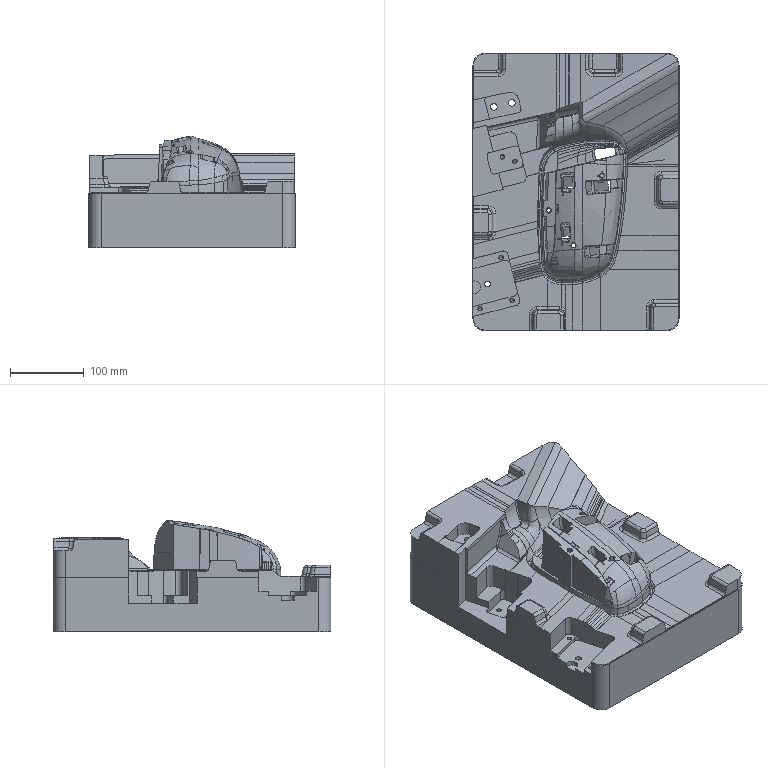Part | STEP file | 车灯-后视镜_id366_x_t | 1 solid | 793 faces | volume 9620612 mm3 | plane 292 | spline 288 | cylinder 137 | other 61 | cone 13 | sphere 1 | torus 1 | commonest cylinder face diameters 6 x41 8 x22 12 x21 10 x10 10.4 x6 5.1 x5